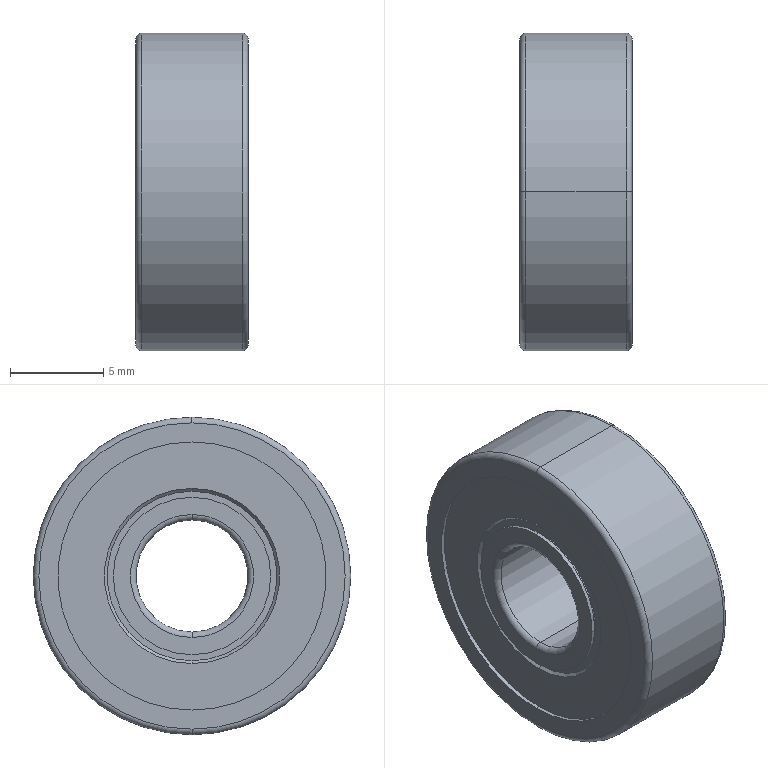Part | SolidWorks | features BaseBody 1 | 1 solid | 98 faces | box 6 x 17 x 17 mm | volume 1023 mm3 | cylinder 40 | torus 24 | cone 20 | plane 14 | commonest cylinder face diameters 8.776 x8 14.354 x8 8 x4 8.216 x4 8.432 x4 9.078 x4